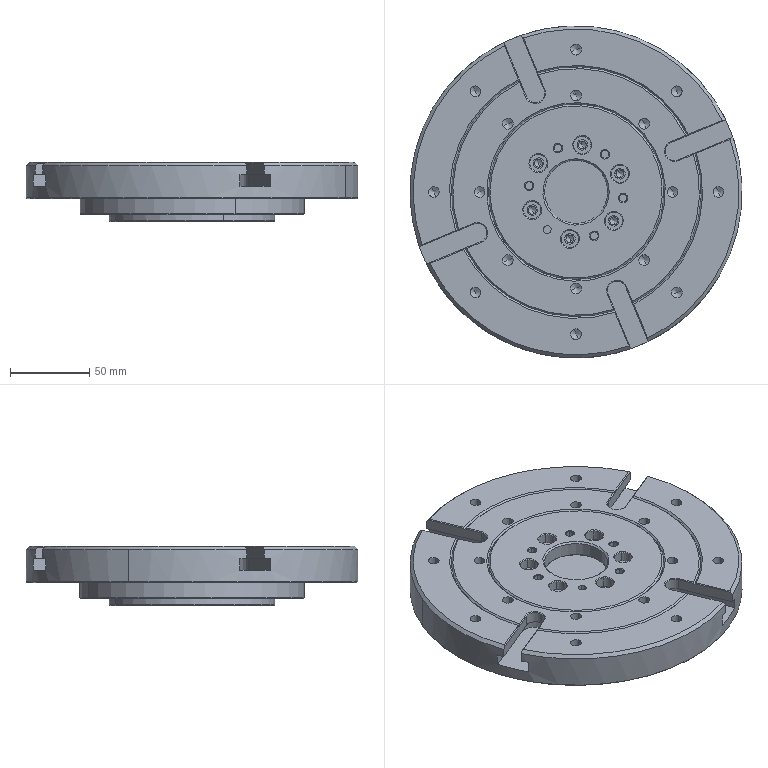CAM job | Mastercam | 3-axis milling, 5-axis milling, drilling
Tools:
tool_number,name,type,diameter_mm,corner_radius_mm,flutes,flute_length_mm,overall_length_mm,shoulder_length_mm,holder_diameter_mm,length_offset,diameter_offset,default_rpm,default_feed_mm_min,default_plunge_mm_min,coolant
1,25 Bull Nose Mill,bull end mill,25,0.8,4,25,75,25,50,1,1,400,48,600,COOL_OFF
1,2 Flat End Mill Rough,end mill,2,0,4,20,20,20,16.002,1,1,5000,600,600,COOL_OFF
1,8 Flat End Mill Rough,end mill,8,0,4,24,24,24,31.877,1,1,6000,4000,2000,COOL_OFF
2,16 Flat End Mill,end mill,16,0,4,50,50,50,50,2,2,625,75,600,COOL_OFF
2,8 Chamfer Mill,chamfer mill,8,0,4,25,25,25,42.012,2,2,3125,375,600,COOL_OFF
2,8 Chamfer Mill,chamfer mill,8,0,4,25,25,25,42.012,2,2,3125,375,600,COOL_OFF
2,2.5 Drill,drill,2.5,0,2,20,20,20,50,2,2,2400,288,600,COOL_OFF
3,2.5 Drill,drill,2.5,0,2,25,50,40,50,3,3,2400,288,600,COOL_OFF
3,10 Chamfer Mill,chamfer mill,10,0,4,25,75,30,50,3,3,2500,300,600,COOL_OFF
3,3.5 Drill,drill,3.5,0,2,25,25,25,42.012,3,3,1714,205.68,600,COOL_OFF
4,8.5 Drill,drill,8.5,0,2,25,50,40,50,4,4,706,84.72,600,COOL_OFF
4,12 Flat End Mill Rough,end mill,12,0,4,25,25,25,42.012,4,4,833,99.96,600,COOL_OFF
5,6 Carbide Chamfer Mill,chamfer mill,6,0,4,25,25,25,50,5,5,4167,500.04,600,COOL_OFF
5,14 Flat End Mill,end mill,14,0,4,25,30,25,50,5,5,714,85.68,600,COOL_OFF
5,6 Flat End Mill,end mill,6,0,4,25,25,25,31.877,5,5,1667,200.04,600,COOL_OFF
5,4 Flat End Mill Rough,end mill,4,0,4,20,20,20,31.877,5,5,2500,300,600,COOL_OFF
6,4 Taper Mill,tap,2,0,4,8,25,8,50,6,6,3000,360,600,COOL_OFF
6,2 Flat End Mill Rough,end mill,2,0,4,15,15,15,31.877,6,6,5000,600,600,COOL_OFF
6,3 Flat End Mill Rough,end mill,3,0,4,20,20,20,31.877,6,6,3333,399.96,600,COOL_OFF
6,6.8 Drill,drill,6.8,0,2,25,50,40,50,6,6,882,105.84,600,COOL_OFF
6,3 Flat End Mill Rough,end mill,3,0,4,20,20,20,31.877,6,6,3333,399.96,600,COOL_OFF
7,M8 x 1.25 RH Tap,drill,8,0,2,30,40,30,50,7,7,750,937.5,600,COOL_OFF
7,3 Flat End Mill Finish,end mill,3,0,4,20,20,20,31.877,7,7,3333,399.96,600,COOL_OFF
7,2 Flat End Mill Finish,end mill,2,0,4,15,15,15,31.877,7,7,5000,600,600,COOL_OFF
7,3 Flat End Mill Finish,end mill,3,0,4,20,20,20,50,7,7,3333,399.96,600,COOL_OFF
8,26 60deg Gear cutter,drill,26,0,4,8,80,8,50,8,8,385,46.2,600,COOL_OFF
8,6 Taper Mill,tap,6,0,4,20,20,20,31.877,8,8,4167,500.04,600,COOL_OFF
8,26 60deg Gear cutter,drill,26,0,4,8,80,8,50,8,8,385,46.2,600,COOL_OFF
9,12 Flat End Mill Finish,end mill,12,0,4,25,25,25,42.012,9,9,833,99.96,600,COOL_OFF
9,8 Flat End Mill Finish,end mill,8,0,4,25,25,25,31.877,9,9,1250,150,600,COOL_OFF
10,50 Insert Cutter,bull end mill,50,0.8,4,25,40,25,50,10,10,400,48,600,COOL_OFF
10,12 R0.8,bull end mill,12,0.8,4,25,50,25,50,10,10,1000,120.0,600,COOL_OFF
11,2.4 Thread Mill,thread mill,2.4,0,4,1.5,30,30,50,11,11,2500,300,600,COOL_OFF
11,2 Flat End Mill Finish,end mill,2,0,4,20,20,20,27.495,11,11,5000,600,600,COOL_OFF
11,3 Flat End Mill,end mill,3,0,4,20,20,20,31.877,11,11,3333,399.96,600,COOL_OFF
12,5 Chamfer Mill,chamfer mill,5,0,4,25,25,25,31.877,12,12,5000,600,600,COOL_OFF
12,5.5 Drill,drill,5.5,0,2,28,28,28,50,12,12,1091,130.92,600,COOL_OFF
13,5.5 Flat drill,drill,5.5,0,2,25,27,27,50,13,13,1091,130.92,600,COOL_OFF
13,2.1 Drill,drill,2.1,0,2,20,20,20,31.877,13,13,2857,342.84,600,COOL_OFF
14,1.95 Thread Mill,thread mill,1.95,0,4,1.35,20,10,31.877,14,14,3077,369.24,600,COOL_OFF
15,2.5 Ball Mill,ball end mill,2.5,1.25,4,5,20,5,50,15,15,4800,576,600,COOL_OFF
16,M3 x 0.5 RH Tap,drill,3,0,2,18,46,18,50,16,16,2000,1000,600,COOL_OFF
18,5.5 Drill,drill,5.5,0,2,25,25,25,31.877,18,18,1091,130.92,600,COOL_OFF
18,3.8 Drill,drill,3.8,0,2,25,25,25,31.877,18,18,1579,189.48,600,COOL_OFF
Operations:
seq,operation,operation_type,tool_number,tool_name,tool_diameter_mm,spindle_rpm,feed_mm_min,plunge_mm_min,retract_mm_min,cycle_time_s,wcs,posted,nc_file
1,Contour (Ramp) - [WCS: Top] - [Tplane: Fx1],Contour,1,8 Flat End Mill Rough,8,2300,3500,2000,1200,52.647,Top,yes,1.nc
2,Surface Finish Flowline - [WCS: Top] - [Tplane: Fx1],MultiSurfaceFinishFlowline,1,8 Flat End Mill Rough,8,3500,2000,2000,50,184.53,Top,yes,1.nc
3,Contour (2D) - [WCS: Top] - [Tplane: Fx1],Contour,1,8 Flat End Mill Rough,8,3500,600,2000,1200,12.893,Top,yes,1.nc
4,Drill/Counterbore - [WCS: Top] - [Tplane: Fx1],Drill,3,3.5 Drill,3.5,2000,100,600,1200,7.094,Top,yes,1.nc
5,Peck Drill - [WCS: Top] - [Tplane: Fx1],Drill,4,12 Flat End Mill Rough,12,1000,120,600,1200,84.722,Top,yes,1.nc
6,Drill/Counterbore - [WCS: Top] - [Tplane: Fx1],Drill,5,4 Flat End Mill Rough,4,700,60,600,1200,49.171,Top,yes,1.nc
7,Peck Drill - [WCS: Top] - [Tplane: Fx1],Drill,6,3 Flat End Mill Rough,3,1200,150,600,1200,11.955,Top,yes,1.nc
8,Drill/Counterbore - [WCS: Top] - [Tplane: Fx1],Drill,3,3.5 Drill,3.5,1000,200,600,1200,1.644,Top,yes,1.nc
9,Tap - [WCS: Top] - [Tplane: Fx1],Drill,7,3 Flat End Mill Finish,3,200,250,600,1200,20.995,Top,yes,1.nc
10,Surface Finish Contour - [WCS: Top] - [Tplane: Fx2],MultiSurfaceFinishContour,1,8 Flat End Mill Rough,8,3500,2000,2000,50,827.269,Top,yes,1.nc
11,Drill/Counterbore - [WCS: Top] - [Tplane: Fx2],Drill,3,3.5 Drill,3.5,2000,100,600,1200,2.285,Top,yes,1.nc
12,Peck Drill - [WCS: Top] - [Tplane: Fx2],Drill,4,12 Flat End Mill Rough,12,1000,120,600,1200,18.642,Top,yes,1.nc
13,Contour (Ramp) - [WCS: Top] - [Tplane: Frt],Contour,10,12 R0.8,12,1600,800,2000,1200,14.038,Top,yes,4.nc
14,Contour (2D) - [WCS: Top] - [Tplane: Frt],Contour,10,12 R0.8,12,1600,400,2000,1200,16.28,Top,yes,4.nc
15,2D High Speed (2D Dynamic Mill) - [WCS: Top] - [Tplane: Frt],HighSpeed2D,4,12 Flat End Mill Rough,12,3000,2000,2000,1200,37.638,Top,yes,4.nc
16,Drill/Counterbore - [WCS: Top] - [Tplane: Frt],Drill,2,2.5 Drill,2.5,2000,100,600,1200,8.64,Top,yes,4.nc
17,Drill/Counterbore - [WCS: Top] - [Tplane: Pl-2],Drill,2,2.5 Drill,2.5,2000,100,600,1200,8.294,Top,yes,4.nc
18,Peck Drill - [WCS: Top] - [Tplane: Frt],Drill,3,3.5 Drill,3.5,2000,60,600,1200,19.67,Top,yes,4.nc
19,Peck Drill - [WCS: Top] - [Tplane: Frt],Drill,3,3.5 Drill,3.5,2000,100,600,1200,5.424,Top,yes,4.nc
20,Drill/Counterbore - [WCS: Top] - [Tplane: Frt],Drill,2,2.5 Drill,2.5,2000,100,600,1200,9.986,Top,yes,4.nc
21,Circle Mill - [WCS: Top] - [Tplane: Frt],CircleMill,6,3 Flat End Mill Rough,3,3500,300,2000,1200,1.972,Top,yes,4.nc
22,Circle Mill - [WCS: Top] - [Tplane: Frt],CircleMill,7,3 Flat End Mill Finish,3,3500,200,2000,1200,4.467,Top,yes,4.nc
23,Contour (2D) - [WCS: Top] - [Tplane: Frt],Contour,9,8 Flat End Mill Finish,8,3500,600,2000,1200,10.569,Top,yes,4.nc
24,Contour (2D chamfer) - [WCS: Top] - [Tplane: Frt],Contour,5,4 Flat End Mill Rough,4,3500,600,2000,1200,6.862,Top,yes,4.nc
25,Contour (2D) - [WCS: Top] - [Tplane: Top],Contour,8,26 60deg Gear cutter,26,4000,1000,2000,1200,18.83,Top,yes,4.nc
26,Contour (2D) - [WCS: Top] - [Tplane: Pl-9],Contour,1,8 Flat End Mill Rough,8,4500,600,2000,1200,29.277,Top,yes,4.nc
27,Contour (2D) - [WCS: Top] - [Tplane: Pl-9],Contour,1,8 Flat End Mill Rough,8,4500,600,2000,1200,2.914,Top,yes,4.nc
28,Contour (2D) - [WCS: Top] - [Tplane: Pl-10],Contour,1,8 Flat End Mill Rough,8,4500,600,2000,1200,29.277,Top,yes,4.nc
29,Contour (2D) - [WCS: Top] - [Tplane: Pl-10],Contour,1,8 Flat End Mill Rough,8,4500,600,2000,1200,2.914,Top,yes,4.nc
30,Peck Drill - [WCS: Top] - [Tplane: Pl-2],Drill,12,5.5 Drill,5.5,2000,80,600,1200,57.294,Top,yes,4.nc
31,Drill/Counterbore - [WCS: Top] - [Tplane: Pl-2],Drill,13,2.1 Drill,2.1,1000,80,600,1200,9.337,Top,yes,4.nc
32,2D High Speed (2D Dynamic Mill) - [WCS: Top] - [Tplane: Top],HighSpeed2D,1,8 Flat End Mill Rough,8,3500,2000,2000,1200,13.392,Top,yes,3.nc
33,2D High Speed (2D Dynamic Mill) - [WCS: Top] - [Tplane: Ins],HighSpeed2D,1,8 Flat End Mill Rough,8,3500,2000,2000,1200,45.151,Top,yes,3.nc
34,2D High Speed (2D Dynamic Mill) - [WCS: Top] - [Tplane: Ins],HighSpeed2D,1,8 Flat End Mill Rough,8,3500,2000,2000,1200,5.942,Top,yes,3.nc
35,Contour (Ramp) - [WCS: Top] - [Tplane: 0d],Contour,1,8 Flat End Mill Rough,8,3500,1000,2000,1200,3.614,Top,yes,3.nc
36,Contour (Ramp) - [WCS: Top] - [Tplane: 30d],Contour,1,8 Flat End Mill Rough,8,3500,1000,2000,1200,3.435,Top,yes,3.nc
37,Contour (Ramp) - [WCS: Top] - [Tplane: 45d],Contour,1,8 Flat End Mill Rough,8,3500,1000,2000,1200,3.494,Top,yes,3.nc
38,Contour (2D) - [WCS: Top] - [Tplane: Out],Contour,1,8 Flat End Mill Rough,8,6000,4000,2000,1200,0.766,Top,yes,3.nc
39,Peck Drill - [WCS: Top] - [Tplane: Out],Drill,2,2.5 Drill,2.5,2000,60,600,1200,11.675,Top,yes,3.nc
40,2D High Speed (2D Dynamic Mill) - [WCS: Top] - [Tplane: Ins-1],HighSpeed2D,1,8 Flat End Mill Rough,8,3500,2000,2000,1200,16.427,Top,yes,3.nc
41,2D High Speed (2D Dynamic Mill) - [WCS: Top] - [Tplane: Ins],HighSpeed2D,1,8 Flat End Mill Rough,8,3500,2000,2000,1200,14.165,Top,yes,3.nc
42,Contour (2D) - [WCS: Top] - [Tplane: Cl],Contour,1,8 Flat End Mill Rough,8,3500,1000,2000,1200,4.041,Top,yes,3.nc
43,Contour (Ramp) - [WCS: Top] - [Tplane: Ins],Contour,5,4 Flat End Mill Rough,4,3500,500,2000,1200,31.198,Top,yes,3.nc
44,Contour (2D) - [WCS: Top] - [Tplane: Ins],Contour,6,3 Flat End Mill Rough,3,5000,600,600,1200,34.207,Top,yes,3.nc
45,Contour (2D) - [WCS: Top] - [Tplane: Top],Contour,9,8 Flat End Mill Finish,8,3500,600,2000,1200,12.274,Top,yes,3.nc
46,Contour (2D) - [WCS: Top] - [Tplane: Ins],Contour,9,8 Flat End Mill Finish,8,3500,600,2000,1200,6.053,Top,yes,3.nc
47,Contour (2D) - [WCS: Top] - [Tplane: Ins],Contour,9,8 Flat End Mill Finish,8,3500,600,2000,1200,7.269,Top,yes,3.nc
48,Contour (2D) - [WCS: Top] - [Tplane: 0d],Contour,9,8 Flat End Mill Finish,8,3500,600,2000,1200,2.058,Top,yes,3.nc
49,Contour (2D) - [WCS: Top] - [Tplane: Cl],Contour,9,8 Flat End Mill Finish,8,3000,400,2000,1200,3.531,Top,yes,3.nc
50,Contour (2D) - [WCS: Top] - [Tplane: 30d],Contour,9,8 Flat End Mill Finish,8,3500,400,2000,1200,2.931,Top,yes,3.nc
51,Contour (2D) - [WCS: Top] - [Tplane: 45d],Contour,9,8 Flat End Mill Finish,8,3500,600,2000,1200,1.919,Top,yes,3.nc
52,Contour (2D) - [WCS: Top] - [Tplane: Ins-1],Contour,9,8 Flat End Mill Finish,8,3500,600,2000,1200,10.098,Top,yes,3.nc
53,Contour (2D) - [WCS: Top] - [Tplane: Ins],Contour,10,12 R0.8,12,3500,400,2000,1200,10.134,Top,yes,3.nc
54,Contour (2D) - [WCS: Top] - [Tplane: Ins],Contour,7,3 Flat End Mill Finish,3,5000,600,2000,1200,7.6,Top,yes,3.nc
55,Contour (2D) - [WCS: Top] - [Tplane: Ins],Contour,7,3 Flat End Mill Finish,3,5000,600,600,1200,7.859,Top,yes,3.nc
56,Contour (2D) - [WCS: Top] - [Tplane: Ins],Contour,7,3 Flat End Mill Finish,3,5000,600,600,1200,7.859,Top,yes,3.nc
57,Contour (2D chamfer) - [WCS: Top] - [Tplane: Ins],Contour,8,26 60deg Gear cutter,26,3000,400,2000,1200,5.272,Top,yes,3.nc
58,Drill/Counterbore - [WCS: Top] - [Tplane: Ins],Drill,12,5.5 Drill,5.5,2000,100,600,1200,1.787,Top,yes,3.nc
59,Peck Drill - [WCS: Top] - [Tplane: Ins],Drill,13,2.1 Drill,2.1,2500,60,600,1200,9.158,Top,yes,3.nc
60,Drill/Counterbore - [WCS: Top] - [Tplane: CB],Drill,11,3 Flat End Mill,3,2000,100,600,1200,2.09,Top,yes,3.nc
61,Thread Mill - [WCS: Top] - [Tplane: Ins],ThreadMill,14,1.95 Thread Mill,1.95,3000,40,2000,1200,108.03,Top,yes,3.nc
62,Deburr 5-axis - [WCS: Top] - [Tplane: Top],459,15,2.5 Ball Mill,2.5,4500,1000,2000,3.581,2.476,Top,yes,3.nc
63,Deburr 5-axis - [WCS: Top] - [Tplane: Top],459,15,2.5 Ball Mill,2.5,4500,1000,2000,3.581,2.981,Top,yes,3.nc
64,Deburr 5-axis - [WCS: Top] - [Tplane: Top],459,15,2.5 Ball Mill,2.5,4500,1000,2000,3.581,3.007,Top,yes,3.nc
65,Drill/Counterbore - [WCS: Top] - [Tplane: Top],Drill,2,2.5 Drill,2.5,2000,100,600,1200,7.887,Top,yes,2.nc
66,Drill/Counterbore - [WCS: Top] - [Tplane: Top],Drill,2,2.5 Drill,2.5,2000,100,600,1200,2.274,Top,yes,2.nc
67,Peck Drill - [WCS: Top] - [Tplane: Top],Drill,3,3.5 Drill,3.5,2000,100,600,1200,34.176,Top,yes,2.nc
68,Tap - [WCS: Top] - [Tplane: Top],Drill,16,M3 x 0.5 RH Tap,3,200,100,600,1200,98.957,Top,yes,2.nc
69,Peck Drill - [WCS: Top] - [Tplane: Top],Drill,18,3.8 Drill,3.8,2000,100,600,1200,6.604,Top,yes,2.nc
70,Circle Mill - [WCS: Top] - [Tplane: Top],CircleMill,6,3 Flat End Mill Rough,3,3500,300,2000,1200,2.077,Top,yes,2.nc
71,Circle Mill - [WCS: Top] - [Tplane: Top],CircleMill,7,3 Flat End Mill Finish,3,3500,200,2000,1200,3.184,Top,yes,2.nc
72,Manual Entry (M00),ManualEntry,,,,0,0,0,0,0,Top,yes,2.nc
73,Contour (2D) - [WCS: Top] - [Tplane: Frt],Contour,8,26 60deg Gear cutter,26,4000,1000,2000,1200,19.225,Top,yes,2.nc
74,Manual Entry (G91 G28 Z0. Y0.),ManualEntry,,,,0,0,0,0,0,Top,yes,2.nc